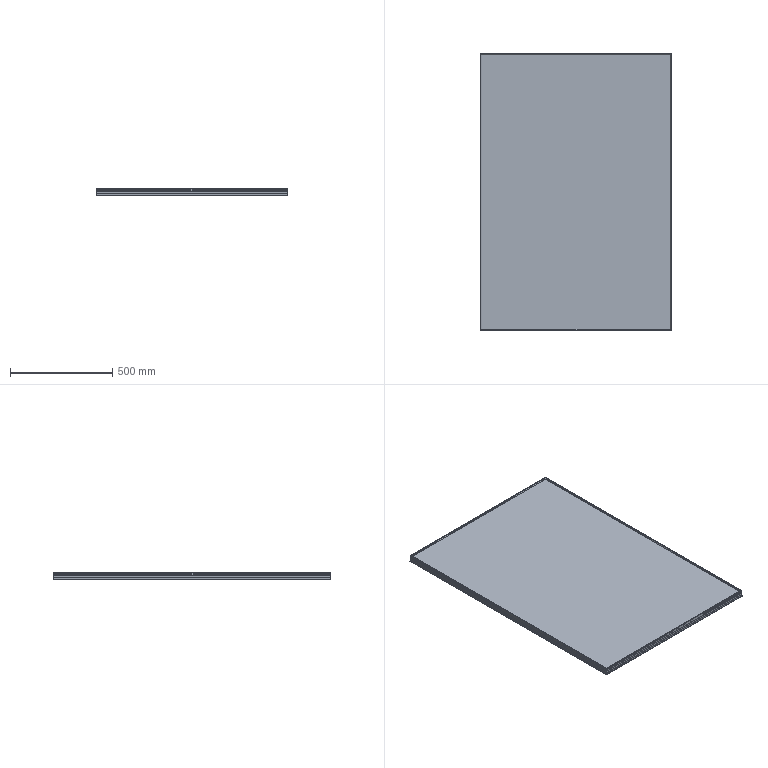Part | SolidWorks | 6 solids | 202 faces | box 940 x 1360 x 36 mm | volume 5509055 mm3 | plane 148 | cylinder 54 | commonest cylinder face diameters 7 x50 5 x4